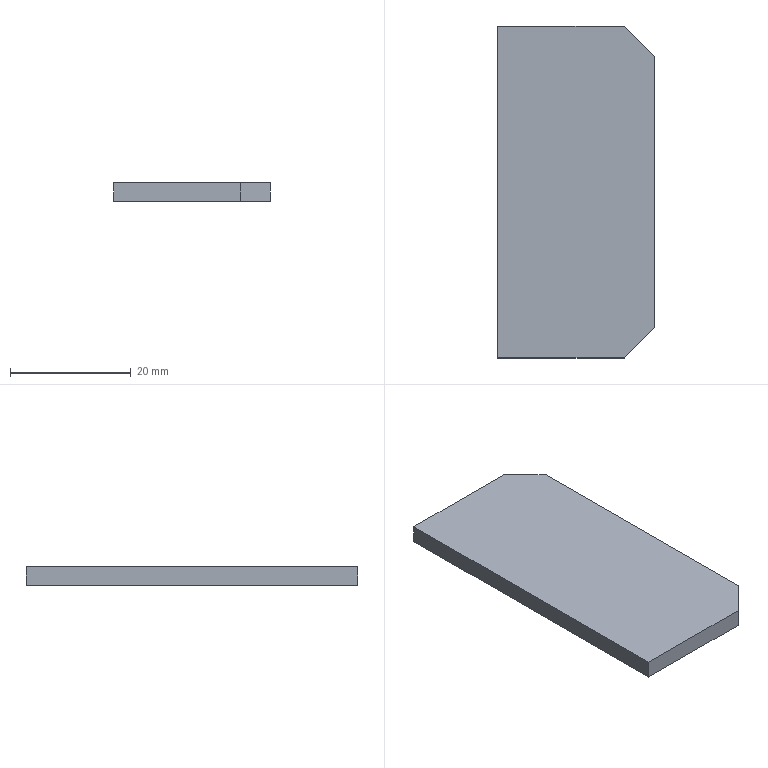Part | 1 solid | 8 faces | box 26 x 55 x 3 mm | volume 4215 mm3 | plane 8
STEP:
#1=CARTESIAN_POINT('',(0.,55.,0.));
#2=VERTEX_POINT('',#1);
#3=CARTESIAN_POINT('',(0.,0.,0.));
#4=VERTEX_POINT('',#3);
#5=CARTESIAN_POINT('',(0.,55.,0.));
#6=DIRECTION('',(0.,-1.,0.));
#7=VECTOR('',#6,1000.);
#8=LINE('',#5,#7);
#9=EDGE_CURVE('',#2,#4,#8,.T.);
#10=ORIENTED_EDGE('',*,*,#9,.T.);
#11=CARTESIAN_POINT('',(0.,0.,3.));
#12=VERTEX_POINT('',#11);
#13=CARTESIAN_POINT('',(0.,0.,3.));
#14=DIRECTION('',(0.,0.,-1.));
#15=VECTOR('',#14,1000.);
#16=LINE('',#13,#15);
#17=EDGE_CURVE('',#12,#4,#16,.T.);
#18=ORIENTED_EDGE('',*,*,#17,.F.);
#19=CARTESIAN_POINT('',(0.,55.,3.));
#20=VERTEX_POINT('',#19);
#21=CARTESIAN_POINT('',(0.,55.,3.));
#22=DIRECTION('',(0.,-1.,0.));
#23=VECTOR('',#22,1000.);
#24=LINE('',#21,#23);
#25=EDGE_CURVE('',#20,#12,#24,.T.);
#26=ORIENTED_EDGE('',*,*,#25,.F.);
#27=CARTESIAN_POINT('',(0.,55.,3.));
#28=DIRECTION('',(0.,0.,-1.));
#29=VECTOR('',#28,1000.);
#30=LINE('',#27,#29);
#31=EDGE_CURVE('',#20,#2,#30,.T.);
#32=ORIENTED_EDGE('',*,*,#31,.T.);
#33=EDGE_LOOP('',(#10,#18,#26,#32));
#34=FACE_OUTER_BOUND('',#33,.T.);
#35=CARTESIAN_POINT('',(0.,55.,3.));
#36=DIRECTION('',(1.,0.,0.));
#37=DIRECTION('',(0.,1.,0.));
#38=AXIS2_PLACEMENT_3D('',#35,#36,#37);
#39=PLANE('',#38);
#40=ADVANCED_FACE('',(#34),#39,.F.);
#41=CARTESIAN_POINT('',(21.,0.,0.));
#42=VERTEX_POINT('',#41);
#43=CARTESIAN_POINT('',(0.,0.,0.));
#44=DIRECTION('',(1.,0.,0.));
#45=VECTOR('',#44,1000.);
#46=LINE('',#43,#45);
#47=EDGE_CURVE('',#4,#42,#46,.T.);
#48=ORIENTED_EDGE('',*,*,#47,.T.);
#49=CARTESIAN_POINT('',(21.,0.,3.));
#50=VERTEX_POINT('',#49);
#51=CARTESIAN_POINT('',(21.,0.,3.));
#52=DIRECTION('',(0.,0.,1.));
#53=VECTOR('',#52,1000.);
#54=LINE('',#51,#53);
#55=EDGE_CURVE('',#42,#50,#54,.T.);
#56=ORIENTED_EDGE('',*,*,#55,.T.);
#57=CARTESIAN_POINT('',(0.,0.,3.));
#58=DIRECTION('',(1.,0.,0.));
#59=VECTOR('',#58,1000.);
#60=LINE('',#57,#59);
#61=EDGE_CURVE('',#12,#50,#60,.T.);
#62=ORIENTED_EDGE('',*,*,#61,.F.);
#63=ORIENTED_EDGE('',*,*,#17,.T.);
#64=EDGE_LOOP('',(#48,#56,#62,#63));
#65=FACE_OUTER_BOUND('',#64,.T.);
#66=CARTESIAN_POINT('',(0.,0.,3.));
#67=DIRECTION('',(0.,1.,0.));
#68=DIRECTION('',(0.,0.,1.));
#69=AXIS2_PLACEMENT_3D('',#66,#67,#68);
#70=PLANE('',#69);
#71=ADVANCED_FACE('',(#65),#70,.F.);
#72=CARTESIAN_POINT('',(26.,5.,3.));
#73=VERTEX_POINT('',#72);
#74=CARTESIAN_POINT('',(26.,50.,3.));
#75=VERTEX_POINT('',#74);
#76=CARTESIAN_POINT('',(26.,0.,3.));
#77=DIRECTION('',(0.,1.,0.));
#78=VECTOR('',#77,1000.);
#79=LINE('',#76,#78);
#80=EDGE_CURVE('',#73,#75,#79,.T.);
#81=ORIENTED_EDGE('',*,*,#80,.F.);
#82=CARTESIAN_POINT('',(26.,5.,0.));
#83=VERTEX_POINT('',#82);
#84=CARTESIAN_POINT('',(26.,5.,3.));
#85=DIRECTION('',(0.,0.,-1.));
#86=VECTOR('',#85,1000.);
#87=LINE('',#84,#86);
#88=EDGE_CURVE('',#73,#83,#87,.T.);
#89=ORIENTED_EDGE('',*,*,#88,.T.);
#90=CARTESIAN_POINT('',(26.,50.,0.));
#91=VERTEX_POINT('',#90);
#92=CARTESIAN_POINT('',(26.,0.,0.));
#93=DIRECTION('',(0.,1.,0.));
#94=VECTOR('',#93,1000.);
#95=LINE('',#92,#94);
#96=EDGE_CURVE('',#83,#91,#95,.T.);
#97=ORIENTED_EDGE('',*,*,#96,.T.);
#98=CARTESIAN_POINT('',(26.,50.,3.));
#99=DIRECTION('',(0.,0.,1.));
#100=VECTOR('',#99,1000.);
#101=LINE('',#98,#100);
#102=EDGE_CURVE('',#91,#75,#101,.T.);
#103=ORIENTED_EDGE('',*,*,#102,.T.);
#104=EDGE_LOOP('',(#81,#89,#97,#103));
#105=FACE_OUTER_BOUND('',#104,.T.);
#106=CARTESIAN_POINT('',(26.,0.,3.));
#107=DIRECTION('',(-1.,0.,0.));
#108=DIRECTION('',(0.,0.,1.));
#109=AXIS2_PLACEMENT_3D('',#106,#107,#108);
#110=PLANE('',#109);
#111=ADVANCED_FACE('',(#105),#110,.F.);
#112=CARTESIAN_POINT('',(21.,55.,3.));
#113=VERTEX_POINT('',#112);
#114=CARTESIAN_POINT('',(26.,55.,3.));
#115=DIRECTION('',(-1.,0.,0.));
#116=VECTOR('',#115,1000.);
#117=LINE('',#114,#116);
#118=EDGE_CURVE('',#113,#20,#117,.T.);
#119=ORIENTED_EDGE('',*,*,#118,.F.);
#120=CARTESIAN_POINT('',(21.,55.,0.));
#121=VERTEX_POINT('',#120);
#122=CARTESIAN_POINT('',(21.,55.,3.));
#123=DIRECTION('',(0.,0.,-1.));
#124=VECTOR('',#123,1000.);
#125=LINE('',#122,#124);
#126=EDGE_CURVE('',#113,#121,#125,.T.);
#127=ORIENTED_EDGE('',*,*,#126,.T.);
#128=CARTESIAN_POINT('',(26.,55.,0.));
#129=DIRECTION('',(-1.,0.,0.));
#130=VECTOR('',#129,1000.);
#131=LINE('',#128,#130);
#132=EDGE_CURVE('',#121,#2,#131,.T.);
#133=ORIENTED_EDGE('',*,*,#132,.T.);
#134=ORIENTED_EDGE('',*,*,#31,.F.);
#135=EDGE_LOOP('',(#119,#127,#133,#134));
#136=FACE_OUTER_BOUND('',#135,.T.);
#137=CARTESIAN_POINT('',(26.,55.,3.));
#138=DIRECTION('',(0.,-1.,0.));
#139=DIRECTION('',(1.,0.,0.));
#140=AXIS2_PLACEMENT_3D('',#137,#138,#139);
#141=PLANE('',#140);
#142=ADVANCED_FACE('',(#136),#141,.F.);
#143=ORIENTED_EDGE('',*,*,#61,.T.);
#144=CARTESIAN_POINT('',(10.5,-10.5,3.));
#145=DIRECTION('',(0.7071,0.7071,0.));
#146=VECTOR('',#145,1000.);
#147=LINE('',#144,#146);
#148=EDGE_CURVE('',#50,#73,#147,.T.);
#149=ORIENTED_EDGE('',*,*,#148,.T.);
#150=ORIENTED_EDGE('',*,*,#80,.T.);
#151=CARTESIAN_POINT('',(38.,38.,3.));
#152=DIRECTION('',(-0.7071,0.7071,0.));
#153=VECTOR('',#152,1000.);
#154=LINE('',#151,#153);
#155=EDGE_CURVE('',#75,#113,#154,.T.);
#156=ORIENTED_EDGE('',*,*,#155,.T.);
#157=ORIENTED_EDGE('',*,*,#118,.T.);
#158=ORIENTED_EDGE('',*,*,#25,.T.);
#159=EDGE_LOOP('',(#143,#149,#150,#156,#157,#158));
#160=FACE_OUTER_BOUND('',#159,.T.);
#161=CARTESIAN_POINT('',(0.,0.,3.));
#162=DIRECTION('',(0.,0.,1.));
#163=DIRECTION('',(1.,0.,0.));
#164=AXIS2_PLACEMENT_3D('',#161,#162,#163);
#165=PLANE('',#164);
#166=ADVANCED_FACE('',(#160),#165,.T.);
#167=ORIENTED_EDGE('',*,*,#96,.F.);
#168=CARTESIAN_POINT('',(26.,5.,0.));
#169=DIRECTION('',(-0.7071,-0.7071,0.));
#170=VECTOR('',#169,1000.);
#171=LINE('',#168,#170);
#172=EDGE_CURVE('',#83,#42,#171,.T.);
#173=ORIENTED_EDGE('',*,*,#172,.T.);
#174=ORIENTED_EDGE('',*,*,#47,.F.);
#175=ORIENTED_EDGE('',*,*,#9,.F.);
#176=ORIENTED_EDGE('',*,*,#132,.F.);
#177=CARTESIAN_POINT('',(21.,55.,0.));
#178=DIRECTION('',(0.7071,-0.7071,0.));
#179=VECTOR('',#178,1000.);
#180=LINE('',#177,#179);
#181=EDGE_CURVE('',#121,#91,#180,.T.);
#182=ORIENTED_EDGE('',*,*,#181,.T.);
#183=EDGE_LOOP('',(#167,#173,#174,#175,#176,#182));
#184=FACE_OUTER_BOUND('',#183,.T.);
#185=CARTESIAN_POINT('',(0.,0.,0.));
#186=DIRECTION('',(0.,0.,1.));
#187=DIRECTION('',(1.,0.,0.));
#188=AXIS2_PLACEMENT_3D('',#185,#186,#187);
#189=PLANE('',#188);
#190=ADVANCED_FACE('',(#184),#189,.F.);
#191=ORIENTED_EDGE('',*,*,#148,.F.);
#192=ORIENTED_EDGE('',*,*,#55,.F.);
#193=ORIENTED_EDGE('',*,*,#172,.F.);
#194=ORIENTED_EDGE('',*,*,#88,.F.);
#195=EDGE_LOOP('',(#191,#192,#193,#194));
#196=FACE_OUTER_BOUND('',#195,.T.);
#197=CARTESIAN_POINT('',(26.,5.,3.));
#198=DIRECTION('',(-0.7071,0.7071,0.));
#199=DIRECTION('',(0.,0.,-1.));
#200=AXIS2_PLACEMENT_3D('',#197,#198,#199);
#201=PLANE('',#200);
#202=ADVANCED_FACE('',(#196),#201,.F.);
#203=ORIENTED_EDGE('',*,*,#155,.F.);
#204=ORIENTED_EDGE('',*,*,#102,.F.);
#205=ORIENTED_EDGE('',*,*,#181,.F.);
#206=ORIENTED_EDGE('',*,*,#126,.F.);
#207=EDGE_LOOP('',(#203,#204,#205,#206));
#208=FACE_OUTER_BOUND('',#207,.T.);
#209=CARTESIAN_POINT('',(21.,55.,3.));
#210=DIRECTION('',(-0.7071,-0.7071,0.));
#211=DIRECTION('',(0.,0.,-1.));
#212=AXIS2_PLACEMENT_3D('',#209,#210,#211);
#213=PLANE('',#212);
#214=ADVANCED_FACE('',(#208),#213,.F.);
#215=CLOSED_SHELL('',(#40,#71,#111,#142,#166,#190,#202,#214));
#216=MANIFOLD_SOLID_BREP('',#215);
#217=CARTESIAN_POINT('',(0.,0.,0.));
#218=DIRECTION('',(0.,0.,1.));
#219=DIRECTION('',(1.,0.,0.));
#220=AXIS2_PLACEMENT_3D('',#217,#218,#219);
#221=(LENGTH_UNIT()NAMED_UNIT(*)SI_UNIT(.MILLI.,.METRE.));
#222=UNCERTAINTY_MEASURE_WITH_UNIT(LENGTH_MEASURE(0.00001),#221,'','');
#223=(NAMED_UNIT(*)PLANE_ANGLE_UNIT()SI_UNIT($,.RADIAN.));
#224=(NAMED_UNIT(*)SI_UNIT($,.STERADIAN.)SOLID_ANGLE_UNIT());
#225=(GEOMETRIC_REPRESENTATION_CONTEXT(3)GLOBAL_UNCERTAINTY_ASSIGNED_CONTEXT((#222))GLOBAL_UNIT_ASSIGNED_CONTEXT((#221,#223,#224))REPRESENTATION_CONTEXT('',''));
#226=ADVANCED_BREP_SHAPE_REPRESENTATION('',(#216,#220),#225);